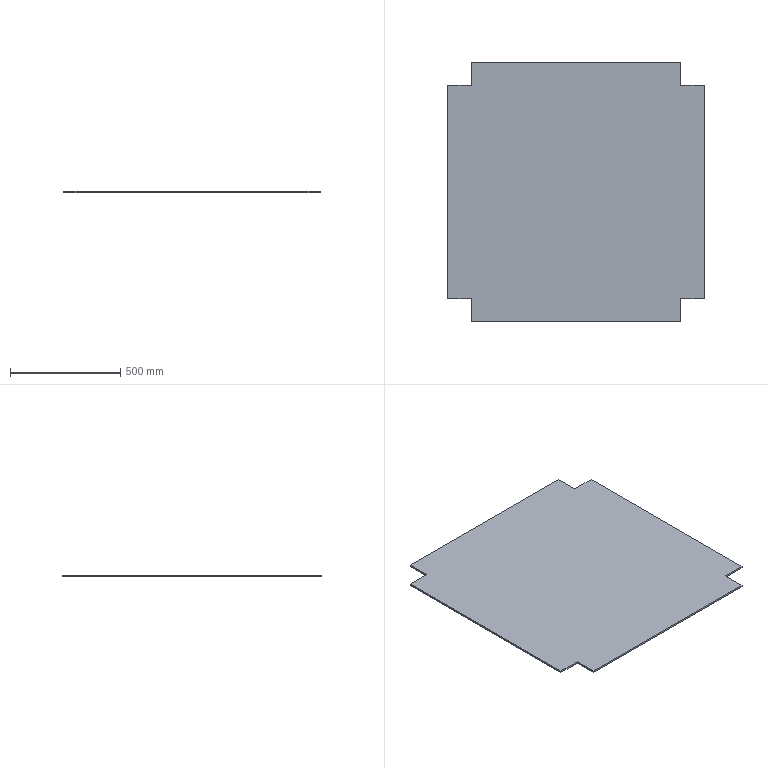Part | SolidWorks | features BaseBody 1 | 1 solid | 14 faces | box 1160 x 1176 x 8 mm | volume 10560480 mm3 | plane 14
STEP:
#1=CARTESIAN_POINT('',(-475.,-588.,0.));
#2=VERTEX_POINT('',#1);
#3=CARTESIAN_POINT('',(475.,-588.,0.));
#4=VERTEX_POINT('',#3);
#5=CARTESIAN_POINT('',(0.,-588.,0.));
#6=DIRECTION('',(1.,0.,0.));
#7=VECTOR('',#6,1000.);
#8=LINE('',#5,#7);
#9=EDGE_CURVE('',#2,#4,#8,.T.);
#10=ORIENTED_EDGE('',*,*,#9,.F.);
#11=CARTESIAN_POINT('',(-475.,-483.,0.));
#12=VERTEX_POINT('',#11);
#13=CARTESIAN_POINT('',(-475.,0.,0.));
#14=DIRECTION('',(0.,-1.,0.));
#15=VECTOR('',#14,1000.);
#16=LINE('',#13,#15);
#17=EDGE_CURVE('',#12,#2,#16,.T.);
#18=ORIENTED_EDGE('',*,*,#17,.F.);
#19=CARTESIAN_POINT('',(-580.,-483.,0.));
#20=VERTEX_POINT('',#19);
#21=CARTESIAN_POINT('',(0.,-483.,0.));
#22=DIRECTION('',(1.,0.,0.));
#23=VECTOR('',#22,1000.);
#24=LINE('',#21,#23);
#25=EDGE_CURVE('',#20,#12,#24,.T.);
#26=ORIENTED_EDGE('',*,*,#25,.F.);
#27=CARTESIAN_POINT('',(-580.,483.,0.));
#28=VERTEX_POINT('',#27);
#29=CARTESIAN_POINT('',(-580.,0.,0.));
#30=DIRECTION('',(0.,-1.,0.));
#31=VECTOR('',#30,1000.);
#32=LINE('',#29,#31);
#33=EDGE_CURVE('',#28,#20,#32,.T.);
#34=ORIENTED_EDGE('',*,*,#33,.F.);
#35=CARTESIAN_POINT('',(-475.,483.,0.));
#36=VERTEX_POINT('',#35);
#37=CARTESIAN_POINT('',(0.,483.,0.));
#38=DIRECTION('',(-1.,0.,0.));
#39=VECTOR('',#38,1000.);
#40=LINE('',#37,#39);
#41=EDGE_CURVE('',#36,#28,#40,.T.);
#42=ORIENTED_EDGE('',*,*,#41,.F.);
#43=CARTESIAN_POINT('',(-475.,588.,0.));
#44=VERTEX_POINT('',#43);
#45=CARTESIAN_POINT('',(-475.,0.,0.));
#46=DIRECTION('',(0.,-1.,0.));
#47=VECTOR('',#46,1000.);
#48=LINE('',#45,#47);
#49=EDGE_CURVE('',#44,#36,#48,.T.);
#50=ORIENTED_EDGE('',*,*,#49,.F.);
#51=CARTESIAN_POINT('',(475.,588.,0.));
#52=VERTEX_POINT('',#51);
#53=CARTESIAN_POINT('',(0.,588.,0.));
#54=DIRECTION('',(-1.,0.,0.));
#55=VECTOR('',#54,1000.);
#56=LINE('',#53,#55);
#57=EDGE_CURVE('',#52,#44,#56,.T.);
#58=ORIENTED_EDGE('',*,*,#57,.F.);
#59=CARTESIAN_POINT('',(475.,483.,0.));
#60=VERTEX_POINT('',#59);
#61=CARTESIAN_POINT('',(475.,0.,0.));
#62=DIRECTION('',(0.,1.,0.));
#63=VECTOR('',#62,1000.);
#64=LINE('',#61,#63);
#65=EDGE_CURVE('',#60,#52,#64,.T.);
#66=ORIENTED_EDGE('',*,*,#65,.F.);
#67=CARTESIAN_POINT('',(580.,483.,0.));
#68=VERTEX_POINT('',#67);
#69=CARTESIAN_POINT('',(0.,483.,0.));
#70=DIRECTION('',(-1.,0.,0.));
#71=VECTOR('',#70,1000.);
#72=LINE('',#69,#71);
#73=EDGE_CURVE('',#68,#60,#72,.T.);
#74=ORIENTED_EDGE('',*,*,#73,.F.);
#75=CARTESIAN_POINT('',(580.,-483.,0.));
#76=VERTEX_POINT('',#75);
#77=CARTESIAN_POINT('',(580.,0.,0.));
#78=DIRECTION('',(0.,1.,0.));
#79=VECTOR('',#78,1000.);
#80=LINE('',#77,#79);
#81=EDGE_CURVE('',#76,#68,#80,.T.);
#82=ORIENTED_EDGE('',*,*,#81,.F.);
#83=CARTESIAN_POINT('',(475.,-483.,0.));
#84=VERTEX_POINT('',#83);
#85=CARTESIAN_POINT('',(0.,-483.,0.));
#86=DIRECTION('',(1.,0.,0.));
#87=VECTOR('',#86,1000.);
#88=LINE('',#85,#87);
#89=EDGE_CURVE('',#84,#76,#88,.T.);
#90=ORIENTED_EDGE('',*,*,#89,.F.);
#91=CARTESIAN_POINT('',(475.,0.,0.));
#92=DIRECTION('',(0.,1.,0.));
#93=VECTOR('',#92,1000.);
#94=LINE('',#91,#93);
#95=EDGE_CURVE('',#4,#84,#94,.T.);
#96=ORIENTED_EDGE('',*,*,#95,.F.);
#97=EDGE_LOOP('',(#10,#18,#26,#34,#42,#50,#58,#66,#74,#82,#90,#96));
#98=FACE_OUTER_BOUND('',#97,.T.);
#99=CARTESIAN_POINT('',(0.,0.,0.));
#100=DIRECTION('',(0.,0.,1.));
#101=DIRECTION('',(1.,0.,0.));
#102=AXIS2_PLACEMENT_3D('',#99,#100,#101);
#103=PLANE('',#102);
#104=ADVANCED_FACE('',(#98),#103,.F.);
#105=CARTESIAN_POINT('',(475.,-483.,8.));
#106=VERTEX_POINT('',#105);
#107=CARTESIAN_POINT('',(475.,-483.,8.));
#108=DIRECTION('',(0.,0.,-1.));
#109=VECTOR('',#108,1000.);
#110=LINE('',#107,#109);
#111=EDGE_CURVE('',#106,#84,#110,.T.);
#112=ORIENTED_EDGE('',*,*,#111,.F.);
#113=CARTESIAN_POINT('',(475.,-588.,8.));
#114=VERTEX_POINT('',#113);
#115=CARTESIAN_POINT('',(475.,0.,8.));
#116=DIRECTION('',(0.,1.,0.));
#117=VECTOR('',#116,1000.);
#118=LINE('',#115,#117);
#119=EDGE_CURVE('',#114,#106,#118,.T.);
#120=ORIENTED_EDGE('',*,*,#119,.F.);
#121=CARTESIAN_POINT('',(475.,-588.,8.));
#122=DIRECTION('',(0.,0.,1.));
#123=VECTOR('',#122,1000.);
#124=LINE('',#121,#123);
#125=EDGE_CURVE('',#4,#114,#124,.T.);
#126=ORIENTED_EDGE('',*,*,#125,.F.);
#127=ORIENTED_EDGE('',*,*,#95,.T.);
#128=EDGE_LOOP('',(#112,#120,#126,#127));
#129=FACE_OUTER_BOUND('',#128,.T.);
#130=CARTESIAN_POINT('',(475.,0.,8.));
#131=DIRECTION('',(-1.,0.,0.));
#132=DIRECTION('',(0.,-1.,0.));
#133=AXIS2_PLACEMENT_3D('',#130,#131,#132);
#134=PLANE('',#133);
#135=ADVANCED_FACE('',(#129),#134,.F.);
#136=CARTESIAN_POINT('',(-475.,-588.,8.));
#137=VERTEX_POINT('',#136);
#138=CARTESIAN_POINT('',(0.,-588.,8.));
#139=DIRECTION('',(-1.,0.,0.));
#140=VECTOR('',#139,1000.);
#141=LINE('',#138,#140);
#142=EDGE_CURVE('',#114,#137,#141,.T.);
#143=ORIENTED_EDGE('',*,*,#142,.T.);
#144=CARTESIAN_POINT('',(-475.,-588.,8.));
#145=DIRECTION('',(0.,0.,-1.));
#146=VECTOR('',#145,1000.);
#147=LINE('',#144,#146);
#148=EDGE_CURVE('',#137,#2,#147,.T.);
#149=ORIENTED_EDGE('',*,*,#148,.T.);
#150=ORIENTED_EDGE('',*,*,#9,.T.);
#151=ORIENTED_EDGE('',*,*,#125,.T.);
#152=EDGE_LOOP('',(#143,#149,#150,#151));
#153=FACE_OUTER_BOUND('',#152,.T.);
#154=CARTESIAN_POINT('',(0.,-588.,8.));
#155=DIRECTION('',(0.,-1.,0.));
#156=DIRECTION('',(1.,0.,0.));
#157=AXIS2_PLACEMENT_3D('',#154,#155,#156);
#158=PLANE('',#157);
#159=ADVANCED_FACE('',(#153),#158,.T.);
#160=ORIENTED_EDGE('',*,*,#148,.F.);
#161=CARTESIAN_POINT('',(-475.,-483.,8.));
#162=VERTEX_POINT('',#161);
#163=CARTESIAN_POINT('',(-475.,0.,8.));
#164=DIRECTION('',(0.,-1.,0.));
#165=VECTOR('',#164,1000.);
#166=LINE('',#163,#165);
#167=EDGE_CURVE('',#162,#137,#166,.T.);
#168=ORIENTED_EDGE('',*,*,#167,.F.);
#169=CARTESIAN_POINT('',(-475.,-483.,8.));
#170=DIRECTION('',(0.,0.,1.));
#171=VECTOR('',#170,1000.);
#172=LINE('',#169,#171);
#173=EDGE_CURVE('',#12,#162,#172,.T.);
#174=ORIENTED_EDGE('',*,*,#173,.F.);
#175=ORIENTED_EDGE('',*,*,#17,.T.);
#176=EDGE_LOOP('',(#160,#168,#174,#175));
#177=FACE_OUTER_BOUND('',#176,.T.);
#178=CARTESIAN_POINT('',(-475.,0.,8.));
#179=DIRECTION('',(1.,0.,0.));
#180=DIRECTION('',(0.,1.,0.));
#181=AXIS2_PLACEMENT_3D('',#178,#179,#180);
#182=PLANE('',#181);
#183=ADVANCED_FACE('',(#177),#182,.F.);
#184=ORIENTED_EDGE('',*,*,#173,.T.);
#185=CARTESIAN_POINT('',(-580.,-483.,8.));
#186=VERTEX_POINT('',#185);
#187=CARTESIAN_POINT('',(0.,-483.,8.));
#188=DIRECTION('',(1.,0.,0.));
#189=VECTOR('',#188,1000.);
#190=LINE('',#187,#189);
#191=EDGE_CURVE('',#186,#162,#190,.T.);
#192=ORIENTED_EDGE('',*,*,#191,.F.);
#193=CARTESIAN_POINT('',(-580.,-483.,8.));
#194=DIRECTION('',(0.,0.,1.));
#195=VECTOR('',#194,1000.);
#196=LINE('',#193,#195);
#197=EDGE_CURVE('',#20,#186,#196,.T.);
#198=ORIENTED_EDGE('',*,*,#197,.F.);
#199=ORIENTED_EDGE('',*,*,#25,.T.);
#200=EDGE_LOOP('',(#184,#192,#198,#199));
#201=FACE_OUTER_BOUND('',#200,.T.);
#202=CARTESIAN_POINT('',(0.,-483.,8.));
#203=DIRECTION('',(0.,1.,0.));
#204=DIRECTION('',(0.,0.,1.));
#205=AXIS2_PLACEMENT_3D('',#202,#203,#204);
#206=PLANE('',#205);
#207=ADVANCED_FACE('',(#201),#206,.F.);
#208=ORIENTED_EDGE('',*,*,#197,.T.);
#209=CARTESIAN_POINT('',(-580.,483.,8.));
#210=VERTEX_POINT('',#209);
#211=CARTESIAN_POINT('',(-580.,0.,8.));
#212=DIRECTION('',(0.,-1.,0.));
#213=VECTOR('',#212,1000.);
#214=LINE('',#211,#213);
#215=EDGE_CURVE('',#210,#186,#214,.T.);
#216=ORIENTED_EDGE('',*,*,#215,.F.);
#217=CARTESIAN_POINT('',(-580.,483.,8.));
#218=DIRECTION('',(0.,0.,1.));
#219=VECTOR('',#218,1000.);
#220=LINE('',#217,#219);
#221=EDGE_CURVE('',#28,#210,#220,.T.);
#222=ORIENTED_EDGE('',*,*,#221,.F.);
#223=ORIENTED_EDGE('',*,*,#33,.T.);
#224=EDGE_LOOP('',(#208,#216,#222,#223));
#225=FACE_OUTER_BOUND('',#224,.T.);
#226=CARTESIAN_POINT('',(-580.,0.,8.));
#227=DIRECTION('',(1.,0.,0.));
#228=DIRECTION('',(0.,0.,-1.));
#229=AXIS2_PLACEMENT_3D('',#226,#227,#228);
#230=PLANE('',#229);
#231=ADVANCED_FACE('',(#225),#230,.F.);
#232=ORIENTED_EDGE('',*,*,#221,.T.);
#233=CARTESIAN_POINT('',(-475.,483.,8.));
#234=VERTEX_POINT('',#233);
#235=CARTESIAN_POINT('',(0.,483.,8.));
#236=DIRECTION('',(-1.,0.,0.));
#237=VECTOR('',#236,1000.);
#238=LINE('',#235,#237);
#239=EDGE_CURVE('',#234,#210,#238,.T.);
#240=ORIENTED_EDGE('',*,*,#239,.F.);
#241=CARTESIAN_POINT('',(-475.,483.,8.));
#242=DIRECTION('',(0.,0.,1.));
#243=VECTOR('',#242,1000.);
#244=LINE('',#241,#243);
#245=EDGE_CURVE('',#36,#234,#244,.T.);
#246=ORIENTED_EDGE('',*,*,#245,.F.);
#247=ORIENTED_EDGE('',*,*,#41,.T.);
#248=EDGE_LOOP('',(#232,#240,#246,#247));
#249=FACE_OUTER_BOUND('',#248,.T.);
#250=CARTESIAN_POINT('',(0.,483.,8.));
#251=DIRECTION('',(0.,-1.,0.));
#252=DIRECTION('',(0.,0.,-1.));
#253=AXIS2_PLACEMENT_3D('',#250,#251,#252);
#254=PLANE('',#253);
#255=ADVANCED_FACE('',(#249),#254,.F.);
#256=ORIENTED_EDGE('',*,*,#245,.T.);
#257=CARTESIAN_POINT('',(-475.,588.,8.));
#258=VERTEX_POINT('',#257);
#259=CARTESIAN_POINT('',(-475.,0.,8.));
#260=DIRECTION('',(0.,-1.,0.));
#261=VECTOR('',#260,1000.);
#262=LINE('',#259,#261);
#263=EDGE_CURVE('',#258,#234,#262,.T.);
#264=ORIENTED_EDGE('',*,*,#263,.F.);
#265=CARTESIAN_POINT('',(-475.,588.,8.));
#266=DIRECTION('',(0.,0.,1.));
#267=VECTOR('',#266,1000.);
#268=LINE('',#265,#267);
#269=EDGE_CURVE('',#44,#258,#268,.T.);
#270=ORIENTED_EDGE('',*,*,#269,.F.);
#271=ORIENTED_EDGE('',*,*,#49,.T.);
#272=EDGE_LOOP('',(#256,#264,#270,#271));
#273=FACE_OUTER_BOUND('',#272,.T.);
#274=CARTESIAN_POINT('',(-475.,0.,8.));
#275=DIRECTION('',(1.,0.,0.));
#276=DIRECTION('',(0.,0.,-1.));
#277=AXIS2_PLACEMENT_3D('',#274,#275,#276);
#278=PLANE('',#277);
#279=ADVANCED_FACE('',(#273),#278,.F.);
#280=ORIENTED_EDGE('',*,*,#269,.T.);
#281=CARTESIAN_POINT('',(475.,588.,8.));
#282=VERTEX_POINT('',#281);
#283=CARTESIAN_POINT('',(0.,588.,8.));
#284=DIRECTION('',(-1.,0.,0.));
#285=VECTOR('',#284,1000.);
#286=LINE('',#283,#285);
#287=EDGE_CURVE('',#282,#258,#286,.T.);
#288=ORIENTED_EDGE('',*,*,#287,.F.);
#289=CARTESIAN_POINT('',(475.,588.,8.));
#290=DIRECTION('',(0.,0.,1.));
#291=VECTOR('',#290,1000.);
#292=LINE('',#289,#291);
#293=EDGE_CURVE('',#52,#282,#292,.T.);
#294=ORIENTED_EDGE('',*,*,#293,.F.);
#295=ORIENTED_EDGE('',*,*,#57,.T.);
#296=EDGE_LOOP('',(#280,#288,#294,#295));
#297=FACE_OUTER_BOUND('',#296,.T.);
#298=CARTESIAN_POINT('',(0.,588.,8.));
#299=DIRECTION('',(0.,-1.,0.));
#300=DIRECTION('',(1.,0.,0.));
#301=AXIS2_PLACEMENT_3D('',#298,#299,#300);
#302=PLANE('',#301);
#303=ADVANCED_FACE('',(#297),#302,.F.);
#304=CARTESIAN_POINT('',(475.,483.,8.));
#305=VERTEX_POINT('',#304);
#306=CARTESIAN_POINT('',(475.,0.,8.));
#307=DIRECTION('',(0.,-1.,0.));
#308=VECTOR('',#307,1000.);
#309=LINE('',#306,#308);
#310=EDGE_CURVE('',#282,#305,#309,.T.);
#311=ORIENTED_EDGE('',*,*,#310,.T.);
#312=CARTESIAN_POINT('',(475.,483.,8.));
#313=DIRECTION('',(0.,0.,-1.));
#314=VECTOR('',#313,1000.);
#315=LINE('',#312,#314);
#316=EDGE_CURVE('',#305,#60,#315,.T.);
#317=ORIENTED_EDGE('',*,*,#316,.T.);
#318=ORIENTED_EDGE('',*,*,#65,.T.);
#319=ORIENTED_EDGE('',*,*,#293,.T.);
#320=EDGE_LOOP('',(#311,#317,#318,#319));
#321=FACE_OUTER_BOUND('',#320,.T.);
#322=CARTESIAN_POINT('',(475.,0.,8.));
#323=DIRECTION('',(1.,0.,0.));
#324=DIRECTION('',(0.,0.,-1.));
#325=AXIS2_PLACEMENT_3D('',#322,#323,#324);
#326=PLANE('',#325);
#327=ADVANCED_FACE('',(#321),#326,.T.);
#328=CARTESIAN_POINT('',(580.,483.,8.));
#329=VERTEX_POINT('',#328);
#330=CARTESIAN_POINT('',(0.,483.,8.));
#331=DIRECTION('',(1.,0.,0.));
#332=VECTOR('',#331,1000.);
#333=LINE('',#330,#332);
#334=EDGE_CURVE('',#305,#329,#333,.T.);
#335=ORIENTED_EDGE('',*,*,#334,.T.);
#336=CARTESIAN_POINT('',(580.,483.,8.));
#337=DIRECTION('',(0.,0.,-1.));
#338=VECTOR('',#337,1000.);
#339=LINE('',#336,#338);
#340=EDGE_CURVE('',#329,#68,#339,.T.);
#341=ORIENTED_EDGE('',*,*,#340,.T.);
#342=ORIENTED_EDGE('',*,*,#73,.T.);
#343=ORIENTED_EDGE('',*,*,#316,.F.);
#344=EDGE_LOOP('',(#335,#341,#342,#343));
#345=FACE_OUTER_BOUND('',#344,.T.);
#346=CARTESIAN_POINT('',(0.,483.,8.));
#347=DIRECTION('',(0.,1.,0.));
#348=DIRECTION('',(0.,0.,1.));
#349=AXIS2_PLACEMENT_3D('',#346,#347,#348);
#350=PLANE('',#349);
#351=ADVANCED_FACE('',(#345),#350,.T.);
#352=CARTESIAN_POINT('',(580.,-483.,8.));
#353=VERTEX_POINT('',#352);
#354=CARTESIAN_POINT('',(580.,0.,8.));
#355=DIRECTION('',(0.,-1.,0.));
#356=VECTOR('',#355,1000.);
#357=LINE('',#354,#356);
#358=EDGE_CURVE('',#329,#353,#357,.T.);
#359=ORIENTED_EDGE('',*,*,#358,.T.);
#360=CARTESIAN_POINT('',(580.,-483.,8.));
#361=DIRECTION('',(0.,0.,-1.));
#362=VECTOR('',#361,1000.);
#363=LINE('',#360,#362);
#364=EDGE_CURVE('',#353,#76,#363,.T.);
#365=ORIENTED_EDGE('',*,*,#364,.T.);
#366=ORIENTED_EDGE('',*,*,#81,.T.);
#367=ORIENTED_EDGE('',*,*,#340,.F.);
#368=EDGE_LOOP('',(#359,#365,#366,#367));
#369=FACE_OUTER_BOUND('',#368,.T.);
#370=CARTESIAN_POINT('',(580.,0.,8.));
#371=DIRECTION('',(1.,0.,0.));
#372=DIRECTION('',(0.,1.,0.));
#373=AXIS2_PLACEMENT_3D('',#370,#371,#372);
#374=PLANE('',#373);
#375=ADVANCED_FACE('',(#369),#374,.T.);
#376=ORIENTED_EDGE('',*,*,#364,.F.);
#377=CARTESIAN_POINT('',(0.,-483.,8.));
#378=DIRECTION('',(1.,0.,0.));
#379=VECTOR('',#378,1000.);
#380=LINE('',#377,#379);
#381=EDGE_CURVE('',#106,#353,#380,.T.);
#382=ORIENTED_EDGE('',*,*,#381,.F.);
#383=ORIENTED_EDGE('',*,*,#111,.T.);
#384=ORIENTED_EDGE('',*,*,#89,.T.);
#385=EDGE_LOOP('',(#376,#382,#383,#384));
#386=FACE_OUTER_BOUND('',#385,.T.);
#387=CARTESIAN_POINT('',(0.,-483.,8.));
#388=DIRECTION('',(0.,1.,0.));
#389=DIRECTION('',(0.,0.,1.));
#390=AXIS2_PLACEMENT_3D('',#387,#388,#389);
#391=PLANE('',#390);
#392=ADVANCED_FACE('',(#386),#391,.F.);
#393=ORIENTED_EDGE('',*,*,#167,.T.);
#394=ORIENTED_EDGE('',*,*,#142,.F.);
#395=ORIENTED_EDGE('',*,*,#119,.T.);
#396=ORIENTED_EDGE('',*,*,#381,.T.);
#397=ORIENTED_EDGE('',*,*,#358,.F.);
#398=ORIENTED_EDGE('',*,*,#334,.F.);
#399=ORIENTED_EDGE('',*,*,#310,.F.);
#400=ORIENTED_EDGE('',*,*,#287,.T.);
#401=ORIENTED_EDGE('',*,*,#263,.T.);
#402=ORIENTED_EDGE('',*,*,#239,.T.);
#403=ORIENTED_EDGE('',*,*,#215,.T.);
#404=ORIENTED_EDGE('',*,*,#191,.T.);
#405=EDGE_LOOP('',(#393,#394,#395,#396,#397,#398,#399,#400,#401,#402,#403,#404));
#406=FACE_OUTER_BOUND('',#405,.T.);
#407=CARTESIAN_POINT('',(0.,0.,8.));
#408=DIRECTION('',(0.,0.,1.));
#409=DIRECTION('',(1.,0.,0.));
#410=AXIS2_PLACEMENT_3D('',#407,#408,#409);
#411=PLANE('',#410);
#412=ADVANCED_FACE('',(#406),#411,.T.);
#413=CLOSED_SHELL('',(#104,#135,#159,#183,#207,#231,#255,#279,#303,#327,#351,#375,#392,#412));
#414=MANIFOLD_SOLID_BREP('',#413);
#415=CARTESIAN_POINT('',(0.,0.,0.));
#416=DIRECTION('',(0.,0.,1.));
#417=DIRECTION('',(1.,0.,0.));
#418=AXIS2_PLACEMENT_3D('',#415,#416,#417);
#419=(LENGTH_UNIT()NAMED_UNIT(*)SI_UNIT(.MILLI.,.METRE.));
#420=UNCERTAINTY_MEASURE_WITH_UNIT(LENGTH_MEASURE(0.00001),#419,'','');
#421=(NAMED_UNIT(*)PLANE_ANGLE_UNIT()SI_UNIT($,.RADIAN.));
#422=(NAMED_UNIT(*)SI_UNIT($,.STERADIAN.)SOLID_ANGLE_UNIT());
#423=(GEOMETRIC_REPRESENTATION_CONTEXT(3)GLOBAL_UNCERTAINTY_ASSIGNED_CONTEXT((#420))GLOBAL_UNIT_ASSIGNED_CONTEXT((#419,#421,#422))REPRESENTATION_CONTEXT('',''));
#424=ADVANCED_BREP_SHAPE_REPRESENTATION('',(#414,#418),#423);